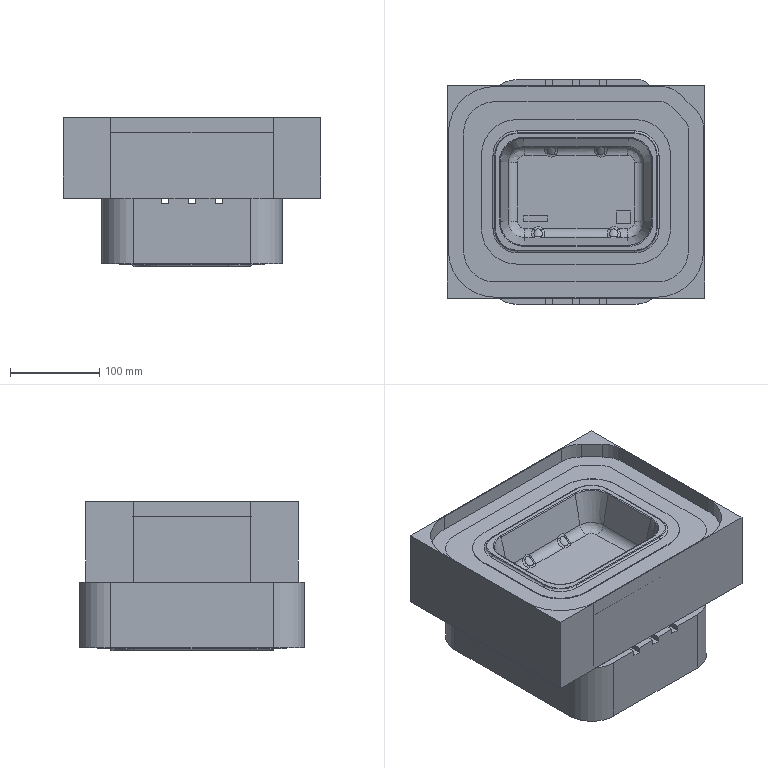Part | 4 solids | 465 faces | box 287.436 x 251.436 x 167.016 mm | volume 7146986 mm3 | plane 226 | cylinder 167 | spline 56 | torus 16 | commonest cylinder face diameters 2 x39 8 x39 21 x16 70 x9 1.39 x8 2.286 x8